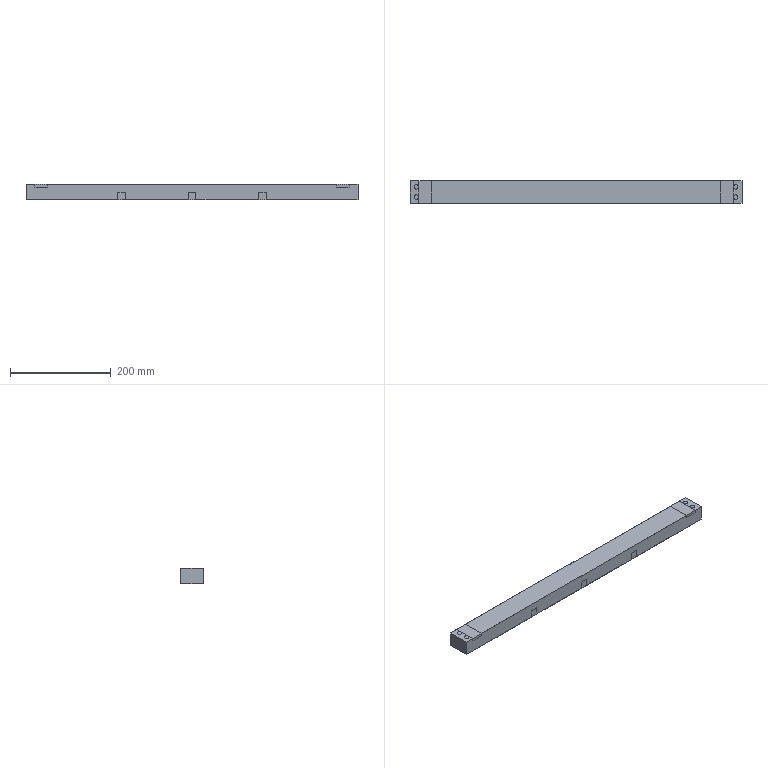NC program | NX | posted with a generic post | part box 659.9 x 45 x 30 mm
Whole program:
N10 G17 G21 G94 G90
(ZLEVEL_PROFILE_COPY_2_1 , TOOL : D50)
N12 T05 M6
N14 G54
N16 G17 G0 G90 X34.343 Y57.239 S6500 M3
N18 G43 Z30. H5
N20 Z-1.938
N22 G94 G1 X27.598 Y53.345 F2000.
N24 G3 X25.098 Y49.015 R5.
N26 G1 Y24.292
N28 X25.1 Y22.545
N30 Y-16.822
N32 X25.098 Y-49.015
N34 G3 X27.597 Y-53.345 R5.
N36 G1 X34.346 Y-57.242
N38 G0 Z-3.875
N40 G1 X27.597 Y-53.345
N42 G2 X25.098 Y-49.015 R5.
N44 G1 X25.1 Y-16.822
N46 Y22.545
N48 X25.098 Y24.292
N50 Y49.015
N52 G2 X27.598 Y53.345 R5.
N54 G1 X34.343 Y57.239
N56 G0 Z-5.813
N58 G1 X27.598 Y53.345
N60 G3 X25.098 Y49.015 R5.
N62 G1 Y24.292
N64 X25.1 Y22.545
N66 Y-16.822
N68 X25.098 Y-49.015
N70 G3 X27.598 Y-53.345 R5.
N72 G1 X34.346 Y-57.242
N74 G0 Z-7.75
N76 G1 X27.598 Y-53.345
N78 G2 X25.098 Y-49.015 R5.
N80 G1 X25.1 Y-16.822
N82 Y22.545
N84 X25.098 Y24.292
N86 Y49.015
N88 G2 X27.598 Y53.345 R5.
N90 G1 X34.343 Y57.239
N92 G0 Y57.24 Z-9.688
N94 G1 X27.598 Y53.345
N96 G3 X25.098 Y49.015 R5.
N98 G1 X25.1 Y22.545
N100 Y-16.822
N102 X25.098 Y-49.015
N104 G3 X27.598 Y-53.345 R5.
N106 G1 X34.346 Y-57.242
N108 G0 Z-11.625
N110 G1 X27.598 Y-53.345
N112 G2 X25.098 Y-49.015 R5.
N114 G1 X25.1 Y-16.822
N116 Y22.545
N118 X25.098 Y49.015
N120 G2 X27.598 Y53.345 R5.
N122 G1 X34.343 Y57.24
N124 G0 Z-13.563
N126 G1 X27.598 Y53.345
N128 G3 X25.098 Y49.015 R5.
N130 G1 X25.1 Y22.545
N132 Y-16.822
N134 X25.098 Y-49.015
N136 G3 X27.598 Y-53.345 R5.
N138 G1 X34.347 Y-57.242
N140 G0 Z-15.5
N142 G1 X27.598 Y-53.345
N144 G2 X25.098 Y-49.015 R5.
N146 G1 X25.1 Y-16.822
N148 Y22.545
N150 X25.098 Y49.015
N152 G2 X27.598 Y53.345 R5.
N154 G1 X34.343 Y57.24
N156 G0 Z-17.438
N158 G1 X27.598 Y53.345
N160 G3 X25.098 Y49.015 R5.
N162 G1 X25.1 Y22.545
N164 Y-16.822
N166 X25.098 Y-49.015
N168 G3 X27.598 Y-53.345 R5.
N170 G1 X34.347 Y-57.242
N172 G0 Z-19.375
N174 G1 X27.598 Y-53.345
N176 G2 X25.098 Y-49.015 R5.
N178 G1 X25.1 Y-16.822
N180 Y22.545
N182 X25.098 Y49.015
N184 G2 X27.598 Y53.345 R5.
N186 G1 X34.344 Y57.24
N188 G0 Z-21.313
N190 G1 X27.598 Y53.345
N192 G3 X25.099 Y49.015 R5.
N194 G1 X25.1 Y22.545
N196 Y-16.822
N198 X25.099 Y-49.015
N200 G3 X27.598 Y-53.345 R5.
N202 G1 X34.347 Y-57.242
N204 G0 Z-23.25
N206 G1 X27.598 Y-53.345
N208 G2 X25.099 Y-49.015 R5.
N210 G1 X25.1 Y-16.822
N212 Y22.545
N214 X25.099 Y49.015
N216 G2 X27.598 Y53.345 R5.
N218 G1 X34.344 Y57.24
N220 G0 Z-25.188
N222 G1 X27.598 Y53.345
N224 G3 X25.099 Y49.015 R5.
N226 G1 X25.1 Y22.545
N228 Y-16.822
N230 X25.099 Y-49.015
N232 G3 X27.598 Y-53.345 R5.
N234 G1 X34.347 Y-57.242
N236 G0 Z-27.125
N238 G1 X27.599 Y-53.345
N240 G2 X25.099 Y-49.015 R5.
N242 G1 X25.1 Y-16.822
N244 Y22.545
N246 X25.099 Y49.015
N248 G2 X27.599 Y53.345 R5.
N250 G1 X34.344 Y57.24
N252 G0 Z-29.063
N254 G1 X27.599 Y53.345
N256 G3 X25.099 Y49.015 R5.
N258 G1 X25.1 Y22.545
N260 Y-16.822
N262 X25.099 Y-49.015
N264 G3 X27.599 Y-53.345 R5.
N266 G1 X34.348 Y-57.242
N268 G0 Z-31.
N270 G1 X27.599 Y-53.345
N272 G2 X25.099 Y-49.015 R5.
N274 G1 X25.1 Y-16.822
N276 Y22.545
N278 X25.099 Y49.015
N280 G2 X27.599 Y53.345 R5.
N282 G1 X34.344 Y57.24
N284 G0 Z30.
N286 M5
N288 M2